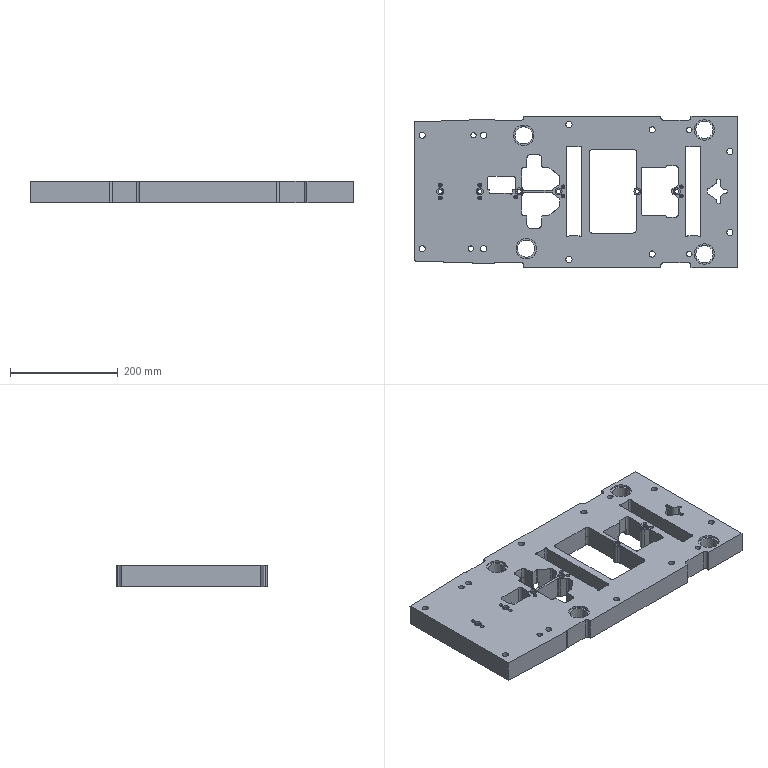Part | NX | features PS-38 2 | 1 solid | 393 faces | box 600 x 280 x 40 mm | volume 4773464 mm3 | cylinder 207 | plane 181 | spline 5 | commonest cylinder face diameters 10 x74 6 x14 6.4 x10 11.5 x10 18 x10 4.001 x9